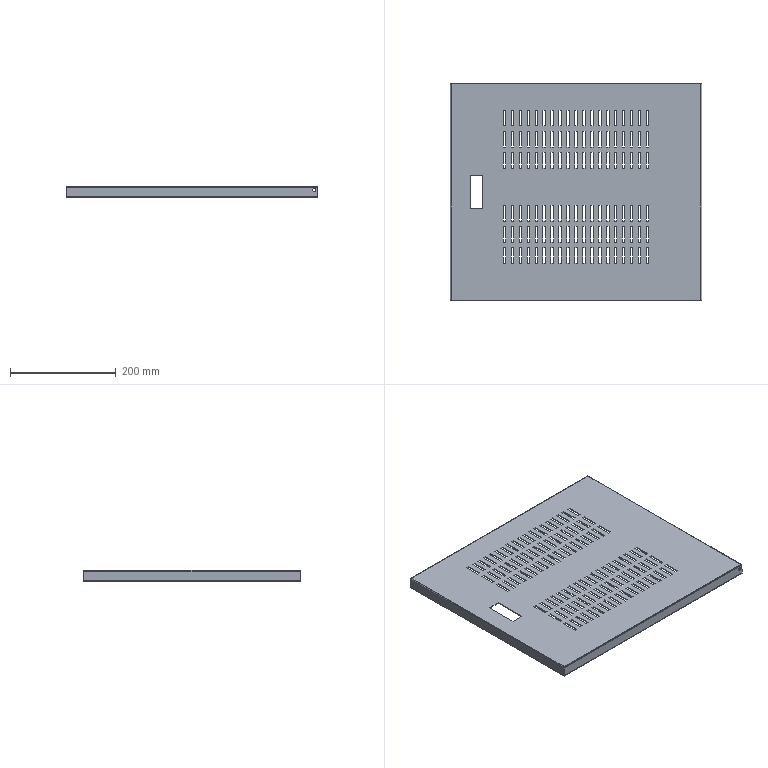Part | SolidWorks | features ICE 3, LPattern 3, EdgeFlange 2, CornerFeat 1, FlatPattern 1, SMBaseFlange 1, SheetMetal 1 | 1 solid | 534 faces | box 476 x 412.001 x 21.5 mm | volume 343155 mm3 | plane 502 | cylinder 20 | spline 12 | commonest cylinder face diameters 0.2 x8 3.2 x8 6 x4